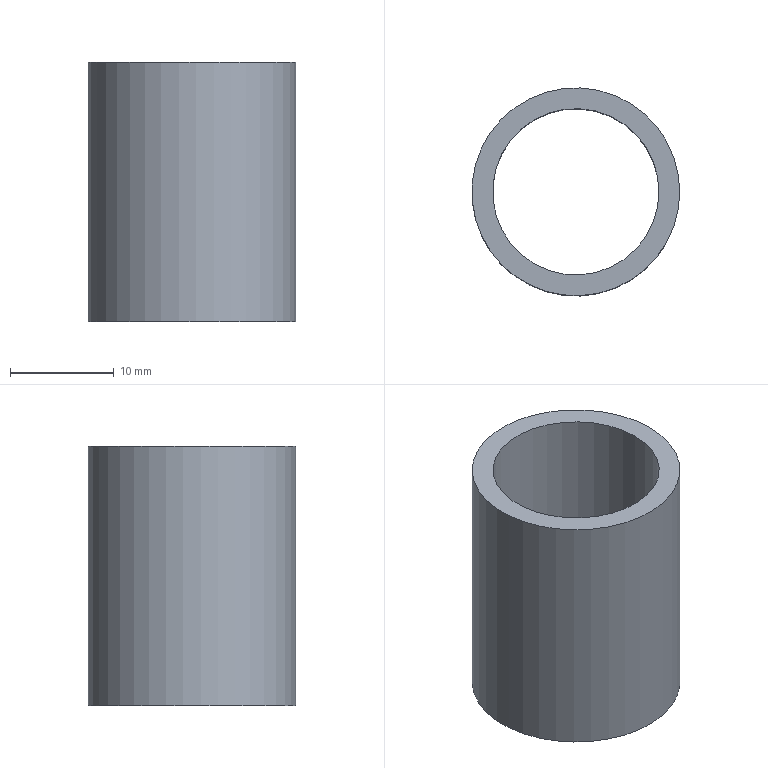Part | STEP file | dingjuguan | 1 solid | 4 faces | box 20 x 20 x 25 mm | volume 2827 mm3 | plane 2 | cylinder 2 | commonest cylinder face diameters 16 x1 20 x1
STEP:
#1=CARTESIAN_POINT('',(0.,0.,0.));
#2=DIRECTION('',(0.,0.,1.));
#3=DIRECTION('',(1.,0.,0.));
#4=AXIS2_PLACEMENT_3D('',#1,#2,#3);
#5=CARTESIAN_POINT('',(10.,0.,12.5));
#6=VERTEX_POINT('',#5);
#7=CARTESIAN_POINT('',(0.,0.,12.5));
#8=DIRECTION('',(0.,0.,1.));
#9=DIRECTION('',(1.,0.,0.));
#10=AXIS2_PLACEMENT_3D('',#7,#8,#9);
#11=CIRCLE('',#10,10.);
#12=CARTESIAN_POINT('',(0.,0.,12.5));
#13=DIRECTION('',(0.,0.,1.));
#14=DIRECTION('',(1.,0.,0.));
#15=AXIS2_PLACEMENT_3D('',#12,#13,#14);
#16=PLANE('',#15);
#17=CARTESIAN_POINT('',(0.,0.));
#18=DIRECTION('',(1.,0.));
#19=AXIS2_PLACEMENT_2D('',#17,#18);
#20=CIRCLE('',#19,10.);
#21=(GEOMETRIC_REPRESENTATION_CONTEXT(2)PARAMETRIC_REPRESENTATION_CONTEXT()REPRESENTATION_CONTEXT('',''));
#22=DEFINITIONAL_REPRESENTATION('',(#20),#21);
#23=PCURVE('',#16,#22);
#24=CARTESIAN_POINT('',(0.,0.,12.5));
#25=DIRECTION('',(0.,0.,-1.));
#26=DIRECTION('',(-1.,0.,0.));
#27=AXIS2_PLACEMENT_3D('',#24,#25,#26);
#28=CYLINDRICAL_SURFACE('',#27,10.);
#29=CARTESIAN_POINT('',(9.425,0.));
#30=DIRECTION('',(-1.,0.));
#31=VECTOR('',#30,1.);
#32=LINE('',#29,#31);
#33=(GEOMETRIC_REPRESENTATION_CONTEXT(2)PARAMETRIC_REPRESENTATION_CONTEXT()REPRESENTATION_CONTEXT('',''));
#34=DEFINITIONAL_REPRESENTATION('',(#32),#33);
#35=PCURVE('',#28,#34);
#36=SURFACE_CURVE('',#11,(#23,#35),.PCURVE_S1.);
#37=EDGE_CURVE('',#6,#6,#36,.T.);
#38=ORIENTED_EDGE('',*,*,#37,.T.);
#39=EDGE_LOOP('',(#38));
#40=FACE_BOUND('',#39,.T.);
#41=CARTESIAN_POINT('',(8.,0.,12.5));
#42=VERTEX_POINT('',#41);
#43=CARTESIAN_POINT('',(0.,0.,12.5));
#44=DIRECTION('',(0.,0.,1.));
#45=DIRECTION('',(1.,0.,0.));
#46=AXIS2_PLACEMENT_3D('',#43,#44,#45);
#47=CIRCLE('',#46,8.);
#48=CARTESIAN_POINT('',(0.,0.));
#49=DIRECTION('',(1.,0.));
#50=AXIS2_PLACEMENT_2D('',#48,#49);
#51=CIRCLE('',#50,8.);
#52=(GEOMETRIC_REPRESENTATION_CONTEXT(2)PARAMETRIC_REPRESENTATION_CONTEXT()REPRESENTATION_CONTEXT('',''));
#53=DEFINITIONAL_REPRESENTATION('',(#51),#52);
#54=PCURVE('',#16,#53);
#55=CARTESIAN_POINT('',(0.,0.,12.5));
#56=DIRECTION('',(0.,0.,-1.));
#57=DIRECTION('',(-1.,0.,0.));
#58=AXIS2_PLACEMENT_3D('',#55,#56,#57);
#59=CYLINDRICAL_SURFACE('',#58,8.);
#60=CARTESIAN_POINT('',(9.425,0.));
#61=DIRECTION('',(-1.,0.));
#62=VECTOR('',#61,1.);
#63=LINE('',#60,#62);
#64=(GEOMETRIC_REPRESENTATION_CONTEXT(2)PARAMETRIC_REPRESENTATION_CONTEXT()REPRESENTATION_CONTEXT('',''));
#65=DEFINITIONAL_REPRESENTATION('',(#63),#64);
#66=PCURVE('',#59,#65);
#67=SURFACE_CURVE('',#47,(#54,#66),.PCURVE_S1.);
#68=EDGE_CURVE('',#42,#42,#67,.T.);
#69=ORIENTED_EDGE('',*,*,#68,.F.);
#70=EDGE_LOOP('',(#69));
#71=FACE_BOUND('',#70,.T.);
#72=ADVANCED_FACE('',(#40,#71),#16,.T.);
#73=CARTESIAN_POINT('',(10.,0.,-12.5));
#74=VERTEX_POINT('',#73);
#75=CARTESIAN_POINT('',(0.,0.,-12.5));
#76=DIRECTION('',(0.,0.,1.));
#77=DIRECTION('',(1.,0.,0.));
#78=AXIS2_PLACEMENT_3D('',#75,#76,#77);
#79=CIRCLE('',#78,10.);
#80=CARTESIAN_POINT('',(0.,0.,-12.5));
#81=DIRECTION('',(0.,0.,1.));
#82=DIRECTION('',(1.,0.,0.));
#83=AXIS2_PLACEMENT_3D('',#80,#81,#82);
#84=PLANE('',#83);
#85=CARTESIAN_POINT('',(0.,0.));
#86=DIRECTION('',(1.,0.));
#87=AXIS2_PLACEMENT_2D('',#85,#86);
#88=CIRCLE('',#87,10.);
#89=(GEOMETRIC_REPRESENTATION_CONTEXT(2)PARAMETRIC_REPRESENTATION_CONTEXT()REPRESENTATION_CONTEXT('',''));
#90=DEFINITIONAL_REPRESENTATION('',(#88),#89);
#91=PCURVE('',#84,#90);
#92=CARTESIAN_POINT('',(9.425,25.));
#93=DIRECTION('',(-1.,0.));
#94=VECTOR('',#93,1.);
#95=LINE('',#92,#94);
#96=(GEOMETRIC_REPRESENTATION_CONTEXT(2)PARAMETRIC_REPRESENTATION_CONTEXT()REPRESENTATION_CONTEXT('',''));
#97=DEFINITIONAL_REPRESENTATION('',(#95),#96);
#98=PCURVE('',#28,#97);
#99=SURFACE_CURVE('',#79,(#91,#98),.PCURVE_S1.);
#100=EDGE_CURVE('',#74,#74,#99,.T.);
#101=ORIENTED_EDGE('',*,*,#100,.F.);
#102=EDGE_LOOP('',(#101));
#103=FACE_BOUND('',#102,.T.);
#104=CARTESIAN_POINT('',(8.,0.,-12.5));
#105=VERTEX_POINT('',#104);
#106=CARTESIAN_POINT('',(0.,0.,-12.5));
#107=DIRECTION('',(0.,0.,1.));
#108=DIRECTION('',(1.,0.,0.));
#109=AXIS2_PLACEMENT_3D('',#106,#107,#108);
#110=CIRCLE('',#109,8.);
#111=CARTESIAN_POINT('',(0.,0.));
#112=DIRECTION('',(1.,0.));
#113=AXIS2_PLACEMENT_2D('',#111,#112);
#114=CIRCLE('',#113,8.);
#115=(GEOMETRIC_REPRESENTATION_CONTEXT(2)PARAMETRIC_REPRESENTATION_CONTEXT()REPRESENTATION_CONTEXT('',''));
#116=DEFINITIONAL_REPRESENTATION('',(#114),#115);
#117=PCURVE('',#84,#116);
#118=CARTESIAN_POINT('',(9.425,25.));
#119=DIRECTION('',(-1.,0.));
#120=VECTOR('',#119,1.);
#121=LINE('',#118,#120);
#122=(GEOMETRIC_REPRESENTATION_CONTEXT(2)PARAMETRIC_REPRESENTATION_CONTEXT()REPRESENTATION_CONTEXT('',''));
#123=DEFINITIONAL_REPRESENTATION('',(#121),#122);
#124=PCURVE('',#59,#123);
#125=SURFACE_CURVE('',#110,(#117,#124),.PCURVE_S1.);
#126=EDGE_CURVE('',#105,#105,#125,.T.);
#127=ORIENTED_EDGE('',*,*,#126,.T.);
#128=EDGE_LOOP('',(#127));
#129=FACE_BOUND('',#128,.T.);
#130=ADVANCED_FACE('',(#103,#129),#84,.F.);
#131=ORIENTED_EDGE('',*,*,#37,.F.);
#132=CARTESIAN_POINT('',(10.,0.,12.5));
#133=CARTESIAN_POINT('',(10.,0.,-12.5));
#134=B_SPLINE_CURVE_WITH_KNOTS('',1,(#132,#133),.UNSPECIFIED.,.F.,.F.,(2,2),(0.,25.),.PIECEWISE_BEZIER_KNOTS.);
#135=CARTESIAN_POINT('',(9.425,0.));
#136=DIRECTION('',(0.,1.));
#137=VECTOR('',#136,1.);
#138=LINE('',#135,#137);
#139=(GEOMETRIC_REPRESENTATION_CONTEXT(2)PARAMETRIC_REPRESENTATION_CONTEXT()REPRESENTATION_CONTEXT('',''));
#140=DEFINITIONAL_REPRESENTATION('',(#138),#139);
#141=PCURVE('',#28,#140);
#142=CARTESIAN_POINT('',(3.142,0.));
#143=DIRECTION('',(0.,1.));
#144=VECTOR('',#143,1.);
#145=LINE('',#142,#144);
#146=(GEOMETRIC_REPRESENTATION_CONTEXT(2)PARAMETRIC_REPRESENTATION_CONTEXT()REPRESENTATION_CONTEXT('',''));
#147=DEFINITIONAL_REPRESENTATION('',(#145),#146);
#148=PCURVE('',#28,#147);
#149=SEAM_CURVE('',#134,(#141,#148),.PCURVE_S1.);
#150=EDGE_CURVE('',#6,#74,#149,.T.);
#151=ORIENTED_EDGE('',*,*,#150,.T.);
#152=ORIENTED_EDGE('',*,*,#100,.T.);
#153=ORIENTED_EDGE('',*,*,#150,.F.);
#154=EDGE_LOOP('',(#131,#151,#152,#153));
#155=FACE_BOUND('',#154,.T.);
#156=ADVANCED_FACE('',(#155),#28,.T.);
#157=ORIENTED_EDGE('',*,*,#68,.F.);
#158=CARTESIAN_POINT('',(8.,0.,12.5));
#159=CARTESIAN_POINT('',(8.,0.,-12.5));
#160=B_SPLINE_CURVE_WITH_KNOTS('',1,(#158,#159),.UNSPECIFIED.,.F.,.F.,(2,2),(0.,25.),.PIECEWISE_BEZIER_KNOTS.);
#161=CARTESIAN_POINT('',(9.425,0.));
#162=DIRECTION('',(0.,1.));
#163=VECTOR('',#162,1.);
#164=LINE('',#161,#163);
#165=(GEOMETRIC_REPRESENTATION_CONTEXT(2)PARAMETRIC_REPRESENTATION_CONTEXT()REPRESENTATION_CONTEXT('',''));
#166=DEFINITIONAL_REPRESENTATION('',(#164),#165);
#167=PCURVE('',#59,#166);
#168=CARTESIAN_POINT('',(3.142,0.));
#169=DIRECTION('',(0.,1.));
#170=VECTOR('',#169,1.);
#171=LINE('',#168,#170);
#172=(GEOMETRIC_REPRESENTATION_CONTEXT(2)PARAMETRIC_REPRESENTATION_CONTEXT()REPRESENTATION_CONTEXT('',''));
#173=DEFINITIONAL_REPRESENTATION('',(#171),#172);
#174=PCURVE('',#59,#173);
#175=SEAM_CURVE('',#160,(#167,#174),.PCURVE_S1.);
#176=EDGE_CURVE('',#42,#105,#175,.T.);
#177=ORIENTED_EDGE('',*,*,#176,.T.);
#178=ORIENTED_EDGE('',*,*,#126,.T.);
#179=ORIENTED_EDGE('',*,*,#176,.F.);
#180=EDGE_LOOP('',(#157,#177,#178,#179));
#181=FACE_BOUND('',#180,.F.);
#182=ADVANCED_FACE('',(#181),#59,.F.);
#183=CLOSED_SHELL('',(#72,#130,#156,#182));
#184=MANIFOLD_SOLID_BREP('',#183);
#185=(LENGTH_UNIT()NAMED_UNIT(*)SI_UNIT(.MILLI.,.METRE.));
#186=UNCERTAINTY_MEASURE_WITH_UNIT(LENGTH_MEASURE(0.00001),#185,'','');
#187=(NAMED_UNIT(*)PLANE_ANGLE_UNIT()SI_UNIT($,.RADIAN.));
#188=(NAMED_UNIT(*)SI_UNIT($,.STERADIAN.)SOLID_ANGLE_UNIT());
#189=(GEOMETRIC_REPRESENTATION_CONTEXT(3)GLOBAL_UNCERTAINTY_ASSIGNED_CONTEXT((#186))GLOBAL_UNIT_ASSIGNED_CONTEXT((#185,#187,#188))REPRESENTATION_CONTEXT('',''));
#190=ADVANCED_BREP_SHAPE_REPRESENTATION('',(#4,#184),#189);